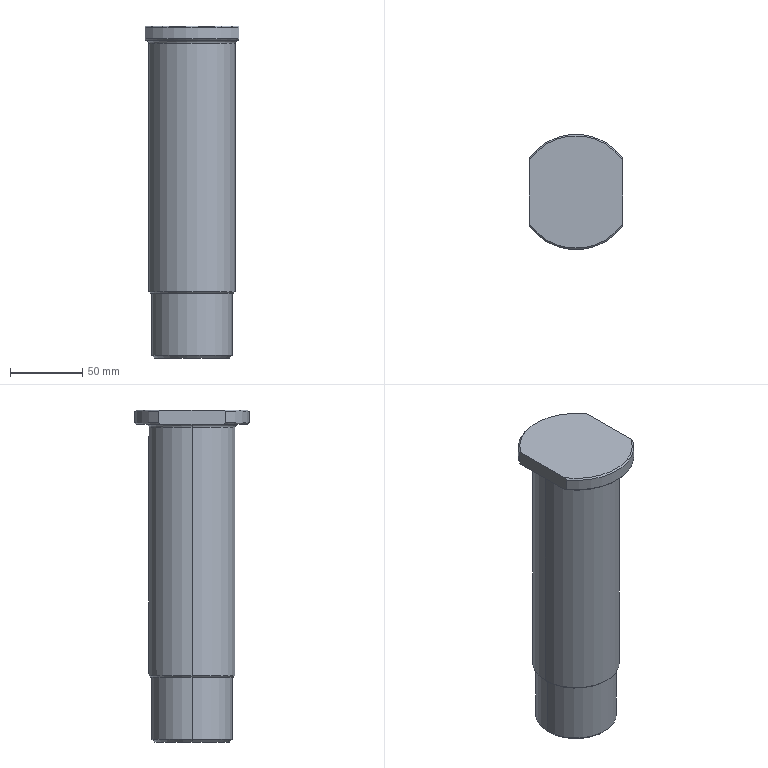Part | SolidWorks | features Chamfer 2, Fillet 2, ICE 2, Revolution 1 | 1 solid | 30 faces | box 65 x 80 x 230 mm | volume 649183 mm3 | cone 10 | cylinder 9 | plane 9 | torus 2 | commonest cylinder face diameters 56 x3 8 x2 60 x2 80 x2
STEP:
#1=CARTESIAN_POINT('',(-32.,0.,-10.));
#2=VERTEX_POINT('',#1);
#3=CARTESIAN_POINT('',(32.,0.,-10.));
#4=VERTEX_POINT('',#3);
#5=CARTESIAN_POINT('',(0.,0.,-10.));
#6=DIRECTION('',(0.,0.,1.));
#7=DIRECTION('',(1.,0.,0.));
#8=AXIS2_PLACEMENT_3D('',#5,#6,#7);
#9=CIRCLE('',#8,32.);
#10=EDGE_CURVE('',#2,#4,#9,.T.);
#11=ORIENTED_EDGE('',*,*,#10,.F.);
#12=CARTESIAN_POINT('',(-30.,0.,-12.));
#13=VERTEX_POINT('',#12);
#14=CARTESIAN_POINT('',(-32.,0.,-12.));
#15=DIRECTION('',(0.,1.,0.));
#16=DIRECTION('',(-1.,0.,0.));
#17=AXIS2_PLACEMENT_3D('',#14,#15,#16);
#18=CIRCLE('',#17,2.);
#19=EDGE_CURVE('',#2,#13,#18,.T.);
#20=ORIENTED_EDGE('',*,*,#19,.T.);
#21=CARTESIAN_POINT('',(30.,0.,-12.));
#22=VERTEX_POINT('',#21);
#23=CARTESIAN_POINT('',(0.,0.,-12.));
#24=DIRECTION('',(0.,0.,-1.));
#25=DIRECTION('',(1.,0.,0.));
#26=AXIS2_PLACEMENT_3D('',#23,#24,#25);
#27=CIRCLE('',#26,30.);
#28=EDGE_CURVE('',#22,#13,#27,.T.);
#29=ORIENTED_EDGE('',*,*,#28,.F.);
#30=CARTESIAN_POINT('',(32.,0.,-12.));
#31=DIRECTION('',(0.,-1.,0.));
#32=DIRECTION('',(0.,0.,-1.));
#33=AXIS2_PLACEMENT_3D('',#30,#31,#32);
#34=CIRCLE('',#33,2.);
#35=EDGE_CURVE('',#4,#22,#34,.T.);
#36=ORIENTED_EDGE('',*,*,#35,.F.);
#37=EDGE_LOOP('',(#11,#20,#29,#36));
#38=FACE_OUTER_BOUND('',#37,.T.);
#39=CARTESIAN_POINT('',(0.,0.,-12.));
#40=DIRECTION('',(0.,0.,1.));
#41=DIRECTION('',(1.,0.,0.));
#42=AXIS2_PLACEMENT_3D('',#39,#40,#41);
#43=TOROIDAL_SURFACE('',#42,32.,2.);
#44=ADVANCED_FACE('',(#38),#43,.F.);
#45=CARTESIAN_POINT('',(-26.,0.,-230.));
#46=VERTEX_POINT('',#45);
#47=CARTESIAN_POINT('',(-4.,25.69,-230.));
#48=VERTEX_POINT('',#47);
#49=CARTESIAN_POINT('',(0.,0.,-230.));
#50=DIRECTION('',(0.,0.,-1.));
#51=DIRECTION('',(1.,0.,0.));
#52=AXIS2_PLACEMENT_3D('',#49,#50,#51);
#53=CIRCLE('',#52,26.);
#54=EDGE_CURVE('',#46,#48,#53,.T.);
#55=ORIENTED_EDGE('',*,*,#54,.F.);
#56=CARTESIAN_POINT('',(-28.,0.,-228.));
#57=VERTEX_POINT('',#56);
#58=CARTESIAN_POINT('',(-28.,0.,-228.));
#59=DIRECTION('',(-0.7071,0.,0.7071));
#60=VECTOR('',#59,1000.);
#61=LINE('',#58,#60);
#62=EDGE_CURVE('',#46,#57,#61,.T.);
#63=ORIENTED_EDGE('',*,*,#62,.T.);
#64=CARTESIAN_POINT('',(-4.,27.713,-228.));
#65=VERTEX_POINT('',#64);
#66=CARTESIAN_POINT('',(0.,0.,-228.));
#67=DIRECTION('',(0.,0.,1.));
#68=DIRECTION('',(1.,0.,0.));
#69=AXIS2_PLACEMENT_3D('',#66,#67,#68);
#70=CIRCLE('',#69,28.);
#71=EDGE_CURVE('',#65,#57,#70,.T.);
#72=ORIENTED_EDGE('',*,*,#71,.F.);
#73=CARTESIAN_POINT('',(-4.,25.69,-230.));
#74=CARTESIAN_POINT('',(-4.,26.365,-229.334));
#75=CARTESIAN_POINT('',(-4.,27.039,-228.667));
#76=CARTESIAN_POINT('',(-4.,27.713,-228.));
#77=B_SPLINE_CURVE_WITH_KNOTS('',3,(#73,#74,#75,#76),.UNSPECIFIED.,.F.,.F.,(4,4),(0.006371,0.009215),.UNSPECIFIED.);
#78=EDGE_CURVE('',#48,#65,#77,.T.);
#79=ORIENTED_EDGE('',*,*,#78,.F.);
#80=EDGE_LOOP('',(#55,#63,#72,#79));
#81=FACE_OUTER_BOUND('',#80,.T.);
#82=CARTESIAN_POINT('',(0.,0.,-228.));
#83=DIRECTION('',(0.,0.,1.));
#84=DIRECTION('',(1.,0.,0.));
#85=AXIS2_PLACEMENT_3D('',#82,#83,#84);
#86=CONICAL_SURFACE('',#85,28.,0.7854);
#87=ADVANCED_FACE('',(#81),#86,.T.);
#88=ORIENTED_EDGE('',*,*,#62,.F.);
#89=CARTESIAN_POINT('',(26.,0.,-230.));
#90=VERTEX_POINT('',#89);
#91=CARTESIAN_POINT('',(0.,0.,-230.));
#92=DIRECTION('',(0.,0.,-1.));
#93=DIRECTION('',(1.,0.,0.));
#94=AXIS2_PLACEMENT_3D('',#91,#92,#93);
#95=CIRCLE('',#94,26.);
#96=EDGE_CURVE('',#90,#46,#95,.T.);
#97=ORIENTED_EDGE('',*,*,#96,.F.);
#98=CARTESIAN_POINT('',(28.,0.,-228.));
#99=VERTEX_POINT('',#98);
#100=CARTESIAN_POINT('',(28.,0.,-228.));
#101=DIRECTION('',(0.7071,0.,0.7071));
#102=VECTOR('',#101,1000.);
#103=LINE('',#100,#102);
#104=EDGE_CURVE('',#90,#99,#103,.T.);
#105=ORIENTED_EDGE('',*,*,#104,.T.);
#106=CARTESIAN_POINT('',(0.,0.,-228.));
#107=DIRECTION('',(0.,0.,1.));
#108=DIRECTION('',(1.,0.,0.));
#109=AXIS2_PLACEMENT_3D('',#106,#107,#108);
#110=CIRCLE('',#109,28.);
#111=EDGE_CURVE('',#57,#99,#110,.T.);
#112=ORIENTED_EDGE('',*,*,#111,.F.);
#113=EDGE_LOOP('',(#88,#97,#105,#112));
#114=FACE_OUTER_BOUND('',#113,.T.);
#115=CARTESIAN_POINT('',(0.,0.,-228.));
#116=DIRECTION('',(0.,0.,1.));
#117=DIRECTION('',(1.,0.,0.));
#118=AXIS2_PLACEMENT_3D('',#115,#116,#117);
#119=CONICAL_SURFACE('',#118,28.,0.7854);
#120=ADVANCED_FACE('',(#114),#119,.T.);
#121=CARTESIAN_POINT('',(-29.,0.,-185.));
#122=VERTEX_POINT('',#121);
#123=CARTESIAN_POINT('',(-4.,28.723,-185.));
#124=VERTEX_POINT('',#123);
#125=CARTESIAN_POINT('',(0.,0.,-185.));
#126=DIRECTION('',(0.,0.,-1.));
#127=DIRECTION('',(1.,0.,0.));
#128=AXIS2_PLACEMENT_3D('',#125,#126,#127);
#129=CIRCLE('',#128,29.);
#130=EDGE_CURVE('',#122,#124,#129,.T.);
#131=ORIENTED_EDGE('',*,*,#130,.F.);
#132=CARTESIAN_POINT('',(-30.,0.,-184.));
#133=VERTEX_POINT('',#132);
#134=CARTESIAN_POINT('',(-30.,0.,-184.));
#135=DIRECTION('',(-0.7071,0.,0.7071));
#136=VECTOR('',#135,1000.);
#137=LINE('',#134,#136);
#138=EDGE_CURVE('',#122,#133,#137,.T.);
#139=ORIENTED_EDGE('',*,*,#138,.T.);
#140=CARTESIAN_POINT('',(-3.873,29.749,-184.));
#141=VERTEX_POINT('',#140);
#142=CARTESIAN_POINT('',(0.,0.,-184.));
#143=DIRECTION('',(0.,0.,1.));
#144=DIRECTION('',(1.,0.,0.));
#145=AXIS2_PLACEMENT_3D('',#142,#143,#144);
#146=CIRCLE('',#145,30.);
#147=EDGE_CURVE('',#141,#133,#146,.T.);
#148=ORIENTED_EDGE('',*,*,#147,.F.);
#149=CARTESIAN_POINT('',(-3.873,29.749,-184.));
#150=CARTESIAN_POINT('',(-3.958,29.407,-184.328));
#151=CARTESIAN_POINT('',(-4.,29.065,-184.661));
#152=CARTESIAN_POINT('',(-4.,28.723,-185.));
#153=B_SPLINE_CURVE_WITH_KNOTS('',3,(#149,#150,#151,#152),.UNSPECIFIED.,.F.,.F.,(4,4),(0.,0.001438),.UNSPECIFIED.);
#154=EDGE_CURVE('',#141,#124,#153,.T.);
#155=ORIENTED_EDGE('',*,*,#154,.T.);
#156=EDGE_LOOP('',(#131,#139,#148,#155));
#157=FACE_OUTER_BOUND('',#156,.T.);
#158=CARTESIAN_POINT('',(0.,0.,-184.));
#159=DIRECTION('',(0.,0.,1.));
#160=DIRECTION('',(1.,0.,0.));
#161=AXIS2_PLACEMENT_3D('',#158,#159,#160);
#162=CONICAL_SURFACE('',#161,30.,0.7854);
#163=ADVANCED_FACE('',(#157),#162,.T.);
#164=ORIENTED_EDGE('',*,*,#138,.F.);
#165=CARTESIAN_POINT('',(29.,0.,-185.));
#166=VERTEX_POINT('',#165);
#167=CARTESIAN_POINT('',(0.,0.,-185.));
#168=DIRECTION('',(0.,0.,-1.));
#169=DIRECTION('',(1.,0.,0.));
#170=AXIS2_PLACEMENT_3D('',#167,#168,#169);
#171=CIRCLE('',#170,29.);
#172=EDGE_CURVE('',#166,#122,#171,.T.);
#173=ORIENTED_EDGE('',*,*,#172,.F.);
#174=CARTESIAN_POINT('',(30.,0.,-184.));
#175=VERTEX_POINT('',#174);
#176=CARTESIAN_POINT('',(30.,0.,-184.));
#177=DIRECTION('',(0.7071,0.,0.7071));
#178=VECTOR('',#177,1000.);
#179=LINE('',#176,#178);
#180=EDGE_CURVE('',#166,#175,#179,.T.);
#181=ORIENTED_EDGE('',*,*,#180,.T.);
#182=CARTESIAN_POINT('',(0.,0.,-184.));
#183=DIRECTION('',(0.,0.,1.));
#184=DIRECTION('',(1.,0.,0.));
#185=AXIS2_PLACEMENT_3D('',#182,#183,#184);
#186=CIRCLE('',#185,30.);
#187=EDGE_CURVE('',#133,#175,#186,.T.);
#188=ORIENTED_EDGE('',*,*,#187,.F.);
#189=EDGE_LOOP('',(#164,#173,#181,#188));
#190=FACE_OUTER_BOUND('',#189,.T.);
#191=CARTESIAN_POINT('',(0.,0.,-184.));
#192=DIRECTION('',(0.,0.,1.));
#193=DIRECTION('',(1.,0.,0.));
#194=AXIS2_PLACEMENT_3D('',#191,#192,#193);
#195=CONICAL_SURFACE('',#194,30.,0.7854);
#196=ADVANCED_FACE('',(#190),#195,.T.);
#197=ORIENTED_EDGE('',*,*,#147,.T.);
#198=CARTESIAN_POINT('',(-30.,0.,-10.));
#199=DIRECTION('',(0.,0.,1.));
#200=VECTOR('',#199,1000.);
#201=LINE('',#198,#200);
#202=EDGE_CURVE('',#133,#13,#201,.T.);
#203=ORIENTED_EDGE('',*,*,#202,.T.);
#204=CARTESIAN_POINT('',(0.,0.,-12.));
#205=DIRECTION('',(0.,0.,-1.));
#206=DIRECTION('',(1.,0.,0.));
#207=AXIS2_PLACEMENT_3D('',#204,#205,#206);
#208=CIRCLE('',#207,30.);
#209=EDGE_CURVE('',#13,#22,#208,.T.);
#210=ORIENTED_EDGE('',*,*,#209,.T.);
#211=CARTESIAN_POINT('',(30.,0.,-10.));
#212=DIRECTION('',(0.,0.,1.));
#213=VECTOR('',#212,1000.);
#214=LINE('',#211,#213);
#215=EDGE_CURVE('',#175,#22,#214,.T.);
#216=ORIENTED_EDGE('',*,*,#215,.F.);
#217=CARTESIAN_POINT('',(3.873,29.749,-184.));
#218=VERTEX_POINT('',#217);
#219=CARTESIAN_POINT('',(0.,0.,-184.));
#220=DIRECTION('',(0.,0.,1.));
#221=DIRECTION('',(1.,0.,0.));
#222=AXIS2_PLACEMENT_3D('',#219,#220,#221);
#223=CIRCLE('',#222,30.);
#224=EDGE_CURVE('',#175,#218,#223,.T.);
#225=ORIENTED_EDGE('',*,*,#224,.T.);
#226=CARTESIAN_POINT('',(0.,30.,-181.));
#227=VERTEX_POINT('',#226);
#228=CARTESIAN_POINT('',(3.873,29.749,-184.));
#229=CARTESIAN_POINT('',(3.762,29.763,-183.57));
#230=CARTESIAN_POINT('',(3.585,29.786,-183.171));
#231=CARTESIAN_POINT('',(3.098,29.841,-182.431));
#232=CARTESIAN_POINT('',(2.801,29.871,-182.11));
#233=CARTESIAN_POINT('',(2.102,29.928,-181.568));
#234=CARTESIAN_POINT('',(1.716,29.954,-181.36));
#235=CARTESIAN_POINT('',(1.089,29.981,-181.145));
#236=CARTESIAN_POINT('',(0.8739,29.988,-181.09));
#237=CARTESIAN_POINT('',(0.4412,29.998,-181.018));
#238=CARTESIAN_POINT('',(0.222,30.,-181.));
#239=CARTESIAN_POINT('',(0.,30.,-181.));
#240=B_SPLINE_CURVE_WITH_KNOTS('',3,(#228,#229,#230,#231,#232,#233,#234,#235,#236,#237,#238,#239),.UNSPECIFIED.,.F.,.F.,(4,2,2,2,2,4),(0.,0.001313,0.002626,0.003939,0.004596,0.005252),.UNSPECIFIED.);
#241=EDGE_CURVE('',#218,#227,#240,.T.);
#242=ORIENTED_EDGE('',*,*,#241,.T.);
#243=CARTESIAN_POINT('',(0.,30.,-181.));
#244=CARTESIAN_POINT('',(-0.444,30.,-181.));
#245=CARTESIAN_POINT('',(-0.8757,29.99,-181.072));
#246=CARTESIAN_POINT('',(-1.714,29.954,-181.359));
#247=CARTESIAN_POINT('',(-2.1,29.928,-181.567));
#248=CARTESIAN_POINT('',(-2.799,29.871,-182.108));
#249=CARTESIAN_POINT('',(-3.097,29.841,-182.43));
#250=CARTESIAN_POINT('',(-3.461,29.8,-182.983));
#251=CARTESIAN_POINT('',(-3.567,29.787,-183.177));
#252=CARTESIAN_POINT('',(-3.745,29.765,-183.578));
#253=CARTESIAN_POINT('',(-3.818,29.756,-183.785));
#254=CARTESIAN_POINT('',(-3.873,29.749,-184.));
#255=B_SPLINE_CURVE_WITH_KNOTS('',3,(#243,#244,#245,#246,#247,#248,#249,#250,#251,#252,#253,#254),.UNSPECIFIED.,.F.,.F.,(4,2,2,2,2,4),(0.,0.001313,0.002626,0.003939,0.004596,0.005252),.UNSPECIFIED.);
#256=EDGE_CURVE('',#227,#141,#255,.T.);
#257=ORIENTED_EDGE('',*,*,#256,.T.);
#258=EDGE_LOOP('',(#197,#203,#210,#216,#225,#242,#257));
#259=FACE_OUTER_BOUND('',#258,.T.);
#260=CARTESIAN_POINT('',(0.,0.,-10.));
#261=DIRECTION('',(0.,0.,1.));
#262=DIRECTION('',(1.,0.,0.));
#263=AXIS2_PLACEMENT_3D('',#260,#261,#262);
#264=CYLINDRICAL_SURFACE('',#263,30.);
#265=ADVANCED_FACE('',(#259),#264,.T.);
#266=ORIENTED_EDGE('',*,*,#71,.T.);
#267=CARTESIAN_POINT('',(-28.,0.,-185.));
#268=VERTEX_POINT('',#267);
#269=CARTESIAN_POINT('',(-28.,0.,-10.));
#270=DIRECTION('',(0.,0.,1.));
#271=VECTOR('',#270,1000.);
#272=LINE('',#269,#271);
#273=EDGE_CURVE('',#57,#268,#272,.T.);
#274=ORIENTED_EDGE('',*,*,#273,.T.);
#275=CARTESIAN_POINT('',(-4.,27.713,-185.));
#276=VERTEX_POINT('',#275);
#277=CARTESIAN_POINT('',(0.,0.,-185.));
#278=DIRECTION('',(0.,0.,1.));
#279=DIRECTION('',(1.,0.,0.));
#280=AXIS2_PLACEMENT_3D('',#277,#278,#279);
#281=CIRCLE('',#280,28.);
#282=EDGE_CURVE('',#276,#268,#281,.T.);
#283=ORIENTED_EDGE('',*,*,#282,.F.);
#284=CARTESIAN_POINT('',(-4.,27.713,-10.));
#285=DIRECTION('',(0.,0.,1.));
#286=VECTOR('',#285,1000.);
#287=LINE('',#284,#286);
#288=EDGE_CURVE('',#65,#276,#287,.T.);
#289=ORIENTED_EDGE('',*,*,#288,.F.);
#290=EDGE_LOOP('',(#266,#274,#283,#289));
#291=FACE_OUTER_BOUND('',#290,.T.);
#292=CARTESIAN_POINT('',(0.,0.,-10.));
#293=DIRECTION('',(0.,0.,1.));
#294=DIRECTION('',(1.,0.,0.));
#295=AXIS2_PLACEMENT_3D('',#292,#293,#294);
#296=CYLINDRICAL_SURFACE('',#295,28.);
#297=ADVANCED_FACE('',(#291),#296,.T.);
#298=ORIENTED_EDGE('',*,*,#273,.F.);
#299=ORIENTED_EDGE('',*,*,#111,.T.);
#300=CARTESIAN_POINT('',(28.,0.,-185.));
#301=VERTEX_POINT('',#300);
#302=CARTESIAN_POINT('',(28.,0.,-10.));
#303=DIRECTION('',(0.,0.,1.));
#304=VECTOR('',#303,1000.);
#305=LINE('',#302,#304);
#306=EDGE_CURVE('',#99,#301,#305,.T.);
#307=ORIENTED_EDGE('',*,*,#306,.T.);
#308=CARTESIAN_POINT('',(0.,0.,-185.));
#309=DIRECTION('',(0.,0.,1.));
#310=DIRECTION('',(1.,0.,0.));
#311=AXIS2_PLACEMENT_3D('',#308,#309,#310);
#312=CIRCLE('',#311,28.);
#313=EDGE_CURVE('',#268,#301,#312,.T.);
#314=ORIENTED_EDGE('',*,*,#313,.F.);
#315=EDGE_LOOP('',(#298,#299,#307,#314));
#316=FACE_OUTER_BOUND('',#315,.T.);
#317=CARTESIAN_POINT('',(0.,0.,-10.));
#318=DIRECTION('',(0.,0.,1.));
#319=DIRECTION('',(1.,0.,0.));
#320=AXIS2_PLACEMENT_3D('',#317,#318,#319);
#321=CYLINDRICAL_SURFACE('',#320,28.);
#322=ADVANCED_FACE('',(#316),#321,.T.);
#323=CARTESIAN_POINT('',(0.,0.,-10.));
#324=DIRECTION('',(0.,0.,1.));
#325=DIRECTION('',(1.,0.,0.));
#326=AXIS2_PLACEMENT_3D('',#323,#324,#325);
#327=CIRCLE('',#326,32.);
#328=EDGE_CURVE('',#4,#2,#327,.T.);
#329=ORIENTED_EDGE('',*,*,#328,.T.);
#330=ORIENTED_EDGE('',*,*,#10,.T.);
#331=EDGE_LOOP('',(#329,#330));
#332=FACE_BOUND('',#331,.T.);
#333=CARTESIAN_POINT('',(32.5,-21.558,-10.));
#334=VERTEX_POINT('',#333);
#335=CARTESIAN_POINT('',(-32.5,-21.558,-10.));
#336=VERTEX_POINT('',#335);
#337=CARTESIAN_POINT('',(0.,0.,-10.));
#338=DIRECTION('',(0.,0.,-1.));
#339=DIRECTION('',(1.,0.,0.));
#340=AXIS2_PLACEMENT_3D('',#337,#338,#339);
#341=CIRCLE('',#340,39.);
#342=EDGE_CURVE('',#334,#336,#341,.T.);
#343=ORIENTED_EDGE('',*,*,#342,.T.);
#344=CARTESIAN_POINT('',(-32.5,21.558,-10.));
#345=VERTEX_POINT('',#344);
#346=CARTESIAN_POINT('',(-32.5,0.,-10.));
#347=DIRECTION('',(0.,1.,0.));
#348=VECTOR('',#347,1000.);
#349=LINE('',#346,#348);
#350=EDGE_CURVE('',#336,#345,#349,.T.);
#351=ORIENTED_EDGE('',*,*,#350,.T.);
#352=CARTESIAN_POINT('',(32.5,21.558,-10.));
#353=VERTEX_POINT('',#352);
#354=CARTESIAN_POINT('',(0.,0.,-10.));
#355=DIRECTION('',(0.,0.,-1.));
#356=DIRECTION('',(1.,0.,0.));
#357=AXIS2_PLACEMENT_3D('',#354,#355,#356);
#358=CIRCLE('',#357,39.);
#359=EDGE_CURVE('',#345,#353,#358,.T.);
#360=ORIENTED_EDGE('',*,*,#359,.T.);
#361=CARTESIAN_POINT('',(32.5,0.,-10.));
#362=DIRECTION('',(0.,1.,0.));
#363=VECTOR('',#362,1000.);
#364=LINE('',#361,#363);
#365=EDGE_CURVE('',#334,#353,#364,.T.);
#366=ORIENTED_EDGE('',*,*,#365,.F.);
#367=EDGE_LOOP('',(#343,#351,#360,#366));
#368=FACE_OUTER_BOUND('',#367,.T.);
#369=CARTESIAN_POINT('',(0.,0.,-10.));
#370=DIRECTION('',(0.,0.,1.));
#371=DIRECTION('',(1.,0.,0.));
#372=AXIS2_PLACEMENT_3D('',#369,#370,#371);
#373=PLANE('',#372);
#374=ADVANCED_FACE('',(#332,#368),#373,.F.);
#375=CARTESIAN_POINT('',(-32.5,23.318,-1.));
#376=VERTEX_POINT('',#375);
#377=CARTESIAN_POINT('',(-32.5,23.318,-9.));
#378=VERTEX_POINT('',#377);
#379=CARTESIAN_POINT('',(-32.5,23.318,-10.));
#380=DIRECTION('',(0.,0.,-1.));
#381=VECTOR('',#380,1000.);
#382=LINE('',#379,#381);
#383=EDGE_CURVE('',#376,#378,#382,.T.);
#384=ORIENTED_EDGE('',*,*,#383,.F.);
#385=CARTESIAN_POINT('',(32.5,23.318,-1.));
#386=VERTEX_POINT('',#385);
#387=CARTESIAN_POINT('',(0.,0.,-1.));
#388=DIRECTION('',(0.,0.,-1.));
#389=DIRECTION('',(1.,0.,0.));
#390=AXIS2_PLACEMENT_3D('',#387,#388,#389);
#391=CIRCLE('',#390,40.);
#392=EDGE_CURVE('',#376,#386,#391,.T.);
#393=ORIENTED_EDGE('',*,*,#392,.T.);
#394=CARTESIAN_POINT('',(32.5,23.318,-9.));
#395=VERTEX_POINT('',#394);
#396=CARTESIAN_POINT('',(32.5,23.318,-10.));
#397=DIRECTION('',(0.,0.,-1.));
#398=VECTOR('',#397,1000.);
#399=LINE('',#396,#398);
#400=EDGE_CURVE('',#386,#395,#399,.T.);
#401=ORIENTED_EDGE('',*,*,#400,.T.);
#402=CARTESIAN_POINT('',(0.,0.,-9.));
#403=DIRECTION('',(0.,0.,1.));
#404=DIRECTION('',(1.,0.,0.));
#405=AXIS2_PLACEMENT_3D('',#402,#403,#404);
#406=CIRCLE('',#405,40.);
#407=EDGE_CURVE('',#395,#378,#406,.T.);
#408=ORIENTED_EDGE('',*,*,#407,.T.);
#409=EDGE_LOOP('',(#384,#393,#401,#408));
#410=FACE_OUTER_BOUND('',#409,.T.);
#411=CARTESIAN_POINT('',(0.,0.,-10.));
#412=DIRECTION('',(0.,0.,1.));
#413=DIRECTION('',(1.,0.,0.));
#414=AXIS2_PLACEMENT_3D('',#411,#412,#413);
#415=CYLINDRICAL_SURFACE('',#414,40.);
#416=ADVANCED_FACE('',(#410),#415,.T.);
#417=CARTESIAN_POINT('',(-32.5,-23.318,-9.));
#418=VERTEX_POINT('',#417);
#419=CARTESIAN_POINT('',(-32.5,-23.318,-1.));
#420=VERTEX_POINT('',#419);
#421=CARTESIAN_POINT('',(-32.5,-23.318,-10.));
#422=DIRECTION('',(0.,0.,1.));
#423=VECTOR('',#422,1000.);
#424=LINE('',#421,#423);
#425=EDGE_CURVE('',#418,#420,#424,.T.);
#426=ORIENTED_EDGE('',*,*,#425,.F.);
#427=CARTESIAN_POINT('',(32.5,-23.318,-9.));
#428=VERTEX_POINT('',#427);
#429=CARTESIAN_POINT('',(0.,0.,-9.));
#430=DIRECTION('',(0.,0.,1.));
#431=DIRECTION('',(1.,0.,0.));
#432=AXIS2_PLACEMENT_3D('',#429,#430,#431);
#433=CIRCLE('',#432,40.);
#434=EDGE_CURVE('',#418,#428,#433,.T.);
#435=ORIENTED_EDGE('',*,*,#434,.T.);
#436=CARTESIAN_POINT('',(32.5,-23.318,-1.));
#437=VERTEX_POINT('',#436);
#438=CARTESIAN_POINT('',(32.5,-23.318,-10.));
#439=DIRECTION('',(0.,0.,1.));
#440=VECTOR('',#439,1000.);
#441=LINE('',#438,#440);
#442=EDGE_CURVE('',#428,#437,#441,.T.);
#443=ORIENTED_EDGE('',*,*,#442,.T.);
#444=CARTESIAN_POINT('',(0.,0.,-1.));
#445=DIRECTION('',(0.,0.,-1.));
#446=DIRECTION('',(1.,0.,0.));
#447=AXIS2_PLACEMENT_3D('',#444,#445,#446);
#448=CIRCLE('',#447,40.);
#449=EDGE_CURVE('',#437,#420,#448,.T.);
#450=ORIENTED_EDGE('',*,*,#449,.T.);
#451=EDGE_LOOP('',(#426,#435,#443,#450));
#452=FACE_OUTER_BOUND('',#451,.T.);
#453=CARTESIAN_POINT('',(0.,0.,-10.));
#454=DIRECTION('',(0.,0.,1.));
#455=DIRECTION('',(1.,0.,0.));
#456=AXIS2_PLACEMENT_3D('',#453,#454,#455);
#457=CYLINDRICAL_SURFACE('',#456,40.);
#458=ADVANCED_FACE('',(#452),#457,.T.);
#459=CARTESIAN_POINT('',(-32.5,-21.558,0.));
#460=VERTEX_POINT('',#459);
#461=CARTESIAN_POINT('',(-32.5,21.558,0.));
#462=VERTEX_POINT('',#461);
#463=CARTESIAN_POINT('',(-32.5,0.,0.));
#464=DIRECTION('',(0.,1.,0.));
#465=VECTOR('',#464,1000.);
#466=LINE('',#463,#465);
#467=EDGE_CURVE('',#460,#462,#466,.T.);
#468=ORIENTED_EDGE('',*,*,#467,.F.);
#469=CARTESIAN_POINT('',(32.5,-21.558,0.));
#470=VERTEX_POINT('',#469);
#471=CARTESIAN_POINT('',(0.,0.,0.));
#472=DIRECTION('',(0.,0.,1.));
#473=DIRECTION('',(1.,0.,0.));
#474=AXIS2_PLACEMENT_3D('',#471,#472,#473);
#475=CIRCLE('',#474,39.);
#476=EDGE_CURVE('',#460,#470,#475,.T.);
#477=ORIENTED_EDGE('',*,*,#476,.T.);
#478=CARTESIAN_POINT('',(32.5,21.558,0.));
#479=VERTEX_POINT('',#478);
#480=CARTESIAN_POINT('',(32.5,0.,0.));
#481=DIRECTION('',(0.,1.,0.));
#482=VECTOR('',#481,1000.);
#483=LINE('',#480,#482);
#484=EDGE_CURVE('',#470,#479,#483,.T.);
#485=ORIENTED_EDGE('',*,*,#484,.T.);
#486=CARTESIAN_POINT('',(0.,0.,0.));
#487=DIRECTION('',(0.,0.,1.));
#488=DIRECTION('',(1.,0.,0.));
#489=AXIS2_PLACEMENT_3D('',#486,#487,#488);
#490=CIRCLE('',#489,39.);
#491=EDGE_CURVE('',#479,#462,#490,.T.);
#492=ORIENTED_EDGE('',*,*,#491,.T.);
#493=EDGE_LOOP('',(#468,#477,#485,#492));
#494=FACE_OUTER_BOUND('',#493,.T.);
#495=CARTESIAN_POINT('',(0.,0.,0.));
#496=DIRECTION('',(0.,0.,1.));
#497=DIRECTION('',(1.,0.,0.));
#498=AXIS2_PLACEMENT_3D('',#495,#496,#497);
#499=PLANE('',#498);
#500=ADVANCED_FACE('',(#494),#499,.T.);
#501=CARTESIAN_POINT('',(-32.5,-23.318,-1.));
#502=CARTESIAN_POINT('',(-32.5,-22.735,-0.6597));
#503=CARTESIAN_POINT('',(-32.5,-22.148,-0.3261));
#504=CARTESIAN_POINT('',(-32.5,-21.558,0.));
#505=B_SPLINE_CURVE_WITH_KNOTS('',3,(#501,#502,#503,#504),.UNSPECIFIED.,.F.,.F.,(4,4),(0.000001379,0.002013),.UNSPECIFIED.);
#506=EDGE_CURVE('',#420,#460,#505,.T.);
#507=ORIENTED_EDGE('',*,*,#506,.F.);
#508=ORIENTED_EDGE('',*,*,#449,.F.);
#509=CARTESIAN_POINT('',(32.5,-23.318,-1.));
#510=CARTESIAN_POINT('',(32.5,-22.735,-0.6597));
#511=CARTESIAN_POINT('',(32.5,-22.148,-0.3261));
#512=CARTESIAN_POINT('',(32.5,-21.558,0.));
#513=B_SPLINE_CURVE_WITH_KNOTS('',3,(#509,#510,#511,#512),.UNSPECIFIED.,.F.,.F.,(4,4),(0.000001379,0.002013),.UNSPECIFIED.);
#514=EDGE_CURVE('',#437,#470,#513,.T.);
#515=ORIENTED_EDGE('',*,*,#514,.T.);
#516=ORIENTED_EDGE('',*,*,#476,.F.);
#517=EDGE_LOOP('',(#507,#508,#515,#516));
#518=FACE_OUTER_BOUND('',#517,.T.);
#519=CARTESIAN_POINT('',(0.,0.,0.));
#520=DIRECTION('',(0.,0.,-1.));
#521=DIRECTION('',(-1.,0.,0.));
#522=AXIS2_PLACEMENT_3D('',#519,#520,#521);
#523=CONICAL_SURFACE('',#522,39.,0.7854);
#524=ADVANCED_FACE('',(#518),#523,.T.);
#525=CARTESIAN_POINT('',(-32.5,21.558,0.));
#526=CARTESIAN_POINT('',(-32.5,22.148,-0.3263));
#527=CARTESIAN_POINT('',(-32.5,22.735,-0.6599));
#528=CARTESIAN_POINT('',(-32.5,23.318,-1.));
#529=B_SPLINE_CURVE_WITH_KNOTS('',3,(#525,#526,#527,#528),.UNSPECIFIED.,.F.,.F.,(4,4),(0.04728,0.04929),.UNSPECIFIED.);
#530=EDGE_CURVE('',#462,#376,#529,.T.);
#531=ORIENTED_EDGE('',*,*,#530,.F.);
#532=ORIENTED_EDGE('',*,*,#491,.F.);
#533=CARTESIAN_POINT('',(32.5,21.558,0.));
#534=CARTESIAN_POINT('',(32.5,22.148,-0.3263));
#535=CARTESIAN_POINT('',(32.5,22.735,-0.6599));
#536=CARTESIAN_POINT('',(32.5,23.318,-1.));
#537=B_SPLINE_CURVE_WITH_KNOTS('',3,(#533,#534,#535,#536),.UNSPECIFIED.,.F.,.F.,(4,4),(0.04728,0.04929),.UNSPECIFIED.);
#538=EDGE_CURVE('',#479,#386,#537,.T.);
#539=ORIENTED_EDGE('',*,*,#538,.T.);
#540=ORIENTED_EDGE('',*,*,#392,.F.);
#541=EDGE_LOOP('',(#531,#532,#539,#540));
#542=FACE_OUTER_BOUND('',#541,.T.);
#543=CARTESIAN_POINT('',(0.,0.,0.));
#544=DIRECTION('',(0.,0.,-1.));
#545=DIRECTION('',(-1.,0.,0.));
#546=AXIS2_PLACEMENT_3D('',#543,#544,#545);
#547=CONICAL_SURFACE('',#546,39.,0.7854);
#548=ADVANCED_FACE('',(#542),#547,.T.);
#549=CARTESIAN_POINT('',(-32.5,23.318,-9.));
#550=CARTESIAN_POINT('',(-32.5,22.735,-9.34));
#551=CARTESIAN_POINT('',(-32.5,22.148,-9.674));
#552=CARTESIAN_POINT('',(-32.5,21.558,-10.));
#553=B_SPLINE_CURVE_WITH_KNOTS('',3,(#549,#550,#551,#552),.UNSPECIFIED.,.F.,.F.,(4,4),(0.000001379,0.002013),.UNSPECIFIED.);
#554=EDGE_CURVE('',#378,#345,#553,.T.);
#555=ORIENTED_EDGE('',*,*,#554,.F.);
#556=ORIENTED_EDGE('',*,*,#407,.F.);
#557=CARTESIAN_POINT('',(32.5,23.318,-9.));
#558=CARTESIAN_POINT('',(32.5,22.735,-9.34));
#559=CARTESIAN_POINT('',(32.5,22.148,-9.674));
#560=CARTESIAN_POINT('',(32.5,21.558,-10.));
#561=B_SPLINE_CURVE_WITH_KNOTS('',3,(#557,#558,#559,#560),.UNSPECIFIED.,.F.,.F.,(4,4),(0.000001379,0.002013),.UNSPECIFIED.);
#562=EDGE_CURVE('',#395,#353,#561,.T.);
#563=ORIENTED_EDGE('',*,*,#562,.T.);
#564=ORIENTED_EDGE('',*,*,#359,.F.);
#565=EDGE_LOOP('',(#555,#556,#563,#564));
#566=FACE_OUTER_BOUND('',#565,.T.);
#567=CARTESIAN_POINT('',(0.,0.,-9.));
#568=DIRECTION('',(0.,0.,1.));
#569=DIRECTION('',(1.,0.,0.));
#570=AXIS2_PLACEMENT_3D('',#567,#568,#569);
#571=CONICAL_SURFACE('',#570,40.,0.7854);
#572=ADVANCED_FACE('',(#566),#571,.T.);
#573=CARTESIAN_POINT('',(-32.5,-21.558,-10.));
#574=CARTESIAN_POINT('',(-32.5,-22.148,-9.674));
#575=CARTESIAN_POINT('',(-32.5,-22.735,-9.34));
#576=CARTESIAN_POINT('',(-32.5,-23.318,-9.));
#577=B_SPLINE_CURVE_WITH_KNOTS('',3,(#573,#574,#575,#576),.UNSPECIFIED.,.F.,.F.,(4,4),(0.04728,0.04929),.UNSPECIFIED.);
#578=EDGE_CURVE('',#336,#418,#577,.T.);
#579=ORIENTED_EDGE('',*,*,#578,.F.);
#580=ORIENTED_EDGE('',*,*,#342,.F.);
#581=CARTESIAN_POINT('',(32.5,-21.558,-10.));
#582=CARTESIAN_POINT('',(32.5,-22.148,-9.674));
#583=CARTESIAN_POINT('',(32.5,-22.735,-9.34));
#584=CARTESIAN_POINT('',(32.5,-23.318,-9.));
#585=B_SPLINE_CURVE_WITH_KNOTS('',3,(#581,#582,#583,#584),.UNSPECIFIED.,.F.,.F.,(4,4),(0.04728,0.04929),.UNSPECIFIED.);
#586=EDGE_CURVE('',#334,#428,#585,.T.);
#587=ORIENTED_EDGE('',*,*,#586,.T.);
#588=ORIENTED_EDGE('',*,*,#434,.F.);
#589=EDGE_LOOP('',(#579,#580,#587,#588));
#590=FACE_OUTER_BOUND('',#589,.T.);
#591=CARTESIAN_POINT('',(0.,0.,-9.));
#592=DIRECTION('',(0.,0.,1.));
#593=DIRECTION('',(1.,0.,0.));
#594=AXIS2_PLACEMENT_3D('',#591,#592,#593);
#595=CONICAL_SURFACE('',#594,40.,0.7854);
#596=ADVANCED_FACE('',(#590),#595,.T.);
#597=CARTESIAN_POINT('',(4.,24.,-230.));
#598=VERTEX_POINT('',#597);
#599=CARTESIAN_POINT('',(4.,25.69,-230.));
#600=VERTEX_POINT('',#599);
#601=CARTESIAN_POINT('',(4.,24.,-230.));
#602=DIRECTION('',(0.,1.,0.));
#603=VECTOR('',#602,1000.);
#604=LINE('',#601,#603);
#605=EDGE_CURVE('',#598,#600,#604,.T.);
#606=ORIENTED_EDGE('',*,*,#605,.T.);
#607=CARTESIAN_POINT('',(0.,0.,-230.));
#608=DIRECTION('',(0.,0.,-1.));
#609=DIRECTION('',(1.,0.,0.));
#610=AXIS2_PLACEMENT_3D('',#607,#608,#609);
#611=CIRCLE('',#610,26.);
#612=EDGE_CURVE('',#600,#90,#611,.T.);
#613=ORIENTED_EDGE('',*,*,#612,.T.);
#614=ORIENTED_EDGE('',*,*,#96,.T.);
#615=ORIENTED_EDGE('',*,*,#54,.T.);
#616=CARTESIAN_POINT('',(-4.,24.,-230.));
#617=VERTEX_POINT('',#616);
#618=CARTESIAN_POINT('',(-4.,24.,-230.));
#619=DIRECTION('',(0.,1.,0.));
#620=VECTOR('',#619,1000.);
#621=LINE('',#618,#620);
#622=EDGE_CURVE('',#617,#48,#621,.T.);
#623=ORIENTED_EDGE('',*,*,#622,.F.);
#624=CARTESIAN_POINT('',(4.,24.,-230.));
#625=DIRECTION('',(-1.,0.,0.));
#626=VECTOR('',#625,1000.);
#627=LINE('',#624,#626);
#628=EDGE_CURVE('',#598,#617,#627,.T.);
#629=ORIENTED_EDGE('',*,*,#628,.F.);
#630=EDGE_LOOP('',(#606,#613,#614,#615,#623,#629));
#631=FACE_OUTER_BOUND('',#630,.T.);
#632=CARTESIAN_POINT('',(0.,0.,-230.));
#633=DIRECTION('',(0.,0.,1.));
#634=DIRECTION('',(1.,0.,0.));
#635=AXIS2_PLACEMENT_3D('',#632,#633,#634);
#636=PLANE('',#635);
#637=ADVANCED_FACE('',(#631),#636,.F.);
#638=ORIENTED_EDGE('',*,*,#306,.F.);
#639=CARTESIAN_POINT('',(4.,27.713,-228.));
#640=VERTEX_POINT('',#639);
#641=CARTESIAN_POINT('',(0.,0.,-228.));
#642=DIRECTION('',(0.,0.,1.));
#643=DIRECTION('',(1.,0.,0.));
#644=AXIS2_PLACEMENT_3D('',#641,#642,#643);
#645=CIRCLE('',#644,28.);
#646=EDGE_CURVE('',#99,#640,#645,.T.);
#647=ORIENTED_EDGE('',*,*,#646,.T.);
#648=CARTESIAN_POINT('',(4.,27.713,-185.));
#649=VERTEX_POINT('',#648);
#650=CARTESIAN_POINT('',(4.,27.713,-10.));
#651=DIRECTION('',(0.,0.,1.));
#652=VECTOR('',#651,1000.);
#653=LINE('',#650,#652);
#654=EDGE_CURVE('',#640,#649,#653,.T.);
#655=ORIENTED_EDGE('',*,*,#654,.T.);
#656=CARTESIAN_POINT('',(0.,0.,-185.));
#657=DIRECTION('',(0.,0.,1.));
#658=DIRECTION('',(1.,0.,0.));
#659=AXIS2_PLACEMENT_3D('',#656,#657,#658);
#660=CIRCLE('',#659,28.);
#661=EDGE_CURVE('',#301,#649,#660,.T.);
#662=ORIENTED_EDGE('',*,*,#661,.F.);
#663=EDGE_LOOP('',(#638,#647,#655,#662));
#664=FACE_OUTER_BOUND('',#663,.T.);
#665=CARTESIAN_POINT('',(0.,0.,-10.));
#666=DIRECTION('',(0.,0.,1.));
#667=DIRECTION('',(1.,0.,0.));
#668=AXIS2_PLACEMENT_3D('',#665,#666,#667);
#669=CYLINDRICAL_SURFACE('',#668,28.);
#670=ADVANCED_FACE('',(#664),#669,.T.);
#671=CARTESIAN_POINT('',(4.,28.723,-185.));
#672=VERTEX_POINT('',#671);
#673=CARTESIAN_POINT('',(4.,0.,-185.));
#674=DIRECTION('',(0.,-1.,0.));
#675=VECTOR('',#674,1000.);
#676=LINE('',#673,#675);
#677=EDGE_CURVE('',#672,#649,#676,.T.);
#678=ORIENTED_EDGE('',*,*,#677,.F.);
#679=CARTESIAN_POINT('',(0.,0.,-185.));
#680=DIRECTION('',(0.,0.,-1.));
#681=DIRECTION('',(1.,0.,0.));
#682=AXIS2_PLACEMENT_3D('',#679,#680,#681);
#683=CIRCLE('',#682,29.);
#684=EDGE_CURVE('',#672,#166,#683,.T.);
#685=ORIENTED_EDGE('',*,*,#684,.T.);
#686=ORIENTED_EDGE('',*,*,#172,.T.);
#687=ORIENTED_EDGE('',*,*,#130,.T.);
#688=CARTESIAN_POINT('',(-4.,0.,-185.));
#689=DIRECTION('',(0.,-1.,0.));
#690=VECTOR('',#689,1000.);
#691=LINE('',#688,#690);
#692=EDGE_CURVE('',#124,#276,#691,.T.);
#693=ORIENTED_EDGE('',*,*,#692,.T.);
#694=ORIENTED_EDGE('',*,*,#282,.T.);
#695=ORIENTED_EDGE('',*,*,#313,.T.);
#696=ORIENTED_EDGE('',*,*,#661,.T.);
#697=EDGE_LOOP('',(#678,#685,#686,#687,#693,#694,#695,#696));
#698=FACE_OUTER_BOUND('',#697,.T.);
#699=CARTESIAN_POINT('',(0.,0.,-185.));
#700=DIRECTION('',(0.,0.,1.));
#701=DIRECTION('',(1.,0.,0.));
#702=AXIS2_PLACEMENT_3D('',#699,#700,#701);
#703=PLANE('',#702);
#704=ADVANCED_FACE('',(#698),#703,.F.);
#705=ORIENTED_EDGE('',*,*,#202,.F.);
#706=ORIENTED_EDGE('',*,*,#187,.T.);
#707=ORIENTED_EDGE('',*,*,#215,.T.);
#708=ORIENTED_EDGE('',*,*,#28,.T.);
#709=EDGE_LOOP('',(#705,#706,#707,#708));
#710=FACE_OUTER_BOUND('',#709,.T.);
#711=CARTESIAN_POINT('',(0.,0.,-10.));
#712=DIRECTION('',(0.,0.,1.));
#713=DIRECTION('',(1.,0.,0.));
#714=AXIS2_PLACEMENT_3D('',#711,#712,#713);
#715=CYLINDRICAL_SURFACE('',#714,30.);
#716=ADVANCED_FACE('',(#710),#715,.T.);
#717=ORIENTED_EDGE('',*,*,#180,.F.);
#718=ORIENTED_EDGE('',*,*,#684,.F.);
#719=CARTESIAN_POINT('',(4.,28.723,-185.));
#720=CARTESIAN_POINT('',(4.,29.065,-184.661));
#721=CARTESIAN_POINT('',(3.958,29.407,-184.328));
#722=CARTESIAN_POINT('',(3.873,29.749,-184.));
#723=B_SPLINE_CURVE_WITH_KNOTS('',3,(#719,#720,#721,#722),.UNSPECIFIED.,.F.,.F.,(4,4),(0.,0.001438),.UNSPECIFIED.);
#724=EDGE_CURVE('',#672,#218,#723,.T.);
#725=ORIENTED_EDGE('',*,*,#724,.T.);
#726=ORIENTED_EDGE('',*,*,#224,.F.);
#727=EDGE_LOOP('',(#717,#718,#725,#726));
#728=FACE_OUTER_BOUND('',#727,.T.);
#729=CARTESIAN_POINT('',(0.,0.,-184.));
#730=DIRECTION('',(0.,0.,1.));
#731=DIRECTION('',(1.,0.,0.));
#732=AXIS2_PLACEMENT_3D('',#729,#730,#731);
#733=CONICAL_SURFACE('',#732,30.,0.7854);
#734=ADVANCED_FACE('',(#728),#733,.T.);
#735=ORIENTED_EDGE('',*,*,#104,.F.);
#736=ORIENTED_EDGE('',*,*,#612,.F.);
#737=CARTESIAN_POINT('',(4.,25.69,-230.));
#738=CARTESIAN_POINT('',(4.,26.365,-229.334));
#739=CARTESIAN_POINT('',(4.,27.039,-228.667));
#740=CARTESIAN_POINT('',(4.,27.713,-228.));
#741=B_SPLINE_CURVE_WITH_KNOTS('',3,(#737,#738,#739,#740),.UNSPECIFIED.,.F.,.F.,(4,4),(0.006371,0.009215),.UNSPECIFIED.);
#742=EDGE_CURVE('',#600,#640,#741,.T.);
#743=ORIENTED_EDGE('',*,*,#742,.T.);
#744=ORIENTED_EDGE('',*,*,#646,.F.);
#745=EDGE_LOOP('',(#735,#736,#743,#744));
#746=FACE_OUTER_BOUND('',#745,.T.);
#747=CARTESIAN_POINT('',(0.,0.,-228.));
#748=DIRECTION('',(0.,0.,1.));
#749=DIRECTION('',(1.,0.,0.));
#750=AXIS2_PLACEMENT_3D('',#747,#748,#749);
#751=CONICAL_SURFACE('',#750,28.,0.7854);
#752=ADVANCED_FACE('',(#746),#751,.T.);
#753=ORIENTED_EDGE('',*,*,#19,.F.);
#754=ORIENTED_EDGE('',*,*,#328,.F.);
#755=ORIENTED_EDGE('',*,*,#35,.T.);
#756=ORIENTED_EDGE('',*,*,#209,.F.);
#757=EDGE_LOOP('',(#753,#754,#755,#756));
#758=FACE_OUTER_BOUND('',#757,.T.);
#759=CARTESIAN_POINT('',(0.,0.,-12.));
#760=DIRECTION('',(0.,0.,1.));
#761=DIRECTION('',(1.,0.,0.));
#762=AXIS2_PLACEMENT_3D('',#759,#760,#761);
#763=TOROIDAL_SURFACE('',#762,32.,2.);
#764=ADVANCED_FACE('',(#758),#763,.F.);
#765=CARTESIAN_POINT('',(-4.,24.,-185.));
#766=VERTEX_POINT('',#765);
#767=CARTESIAN_POINT('',(0.,24.,-181.));
#768=VERTEX_POINT('',#767);
#769=CARTESIAN_POINT('',(0.,24.,-185.));
#770=DIRECTION('',(0.,1.,0.));
#771=DIRECTION('',(0.,0.,-1.));
#772=AXIS2_PLACEMENT_3D('',#769,#770,#771);
#773=CIRCLE('',#772,4.);
#774=EDGE_CURVE('',#766,#768,#773,.T.);
#775=ORIENTED_EDGE('',*,*,#774,.T.);
#776=CARTESIAN_POINT('',(4.,24.,-185.));
#777=VERTEX_POINT('',#776);
#778=CARTESIAN_POINT('',(0.,24.,-185.));
#779=DIRECTION('',(0.,1.,0.));
#780=DIRECTION('',(0.,0.,-1.));
#781=AXIS2_PLACEMENT_3D('',#778,#779,#780);
#782=CIRCLE('',#781,4.);
#783=EDGE_CURVE('',#768,#777,#782,.T.);
#784=ORIENTED_EDGE('',*,*,#783,.T.);
#785=CARTESIAN_POINT('',(4.,24.,-181.));
#786=DIRECTION('',(0.,0.,-1.));
#787=VECTOR('',#786,1000.);
#788=LINE('',#785,#787);
#789=EDGE_CURVE('',#777,#598,#788,.T.);
#790=ORIENTED_EDGE('',*,*,#789,.T.);
#791=ORIENTED_EDGE('',*,*,#628,.T.);
#792=CARTESIAN_POINT('',(-4.,24.,-181.));
#793=DIRECTION('',(0.,0.,-1.));
#794=VECTOR('',#793,1000.);
#795=LINE('',#792,#794);
#796=EDGE_CURVE('',#766,#617,#795,.T.);
#797=ORIENTED_EDGE('',*,*,#796,.F.);
#798=EDGE_LOOP('',(#775,#784,#790,#791,#797));
#799=FACE_OUTER_BOUND('',#798,.T.);
#800=CARTESIAN_POINT('',(4.,24.,-181.));
#801=DIRECTION('',(0.,-1.,0.));
#802=DIRECTION('',(0.,0.,-1.));
#803=AXIS2_PLACEMENT_3D('',#800,#801,#802);
#804=PLANE('',#803);
#805=ADVANCED_FACE('',(#799),#804,.F.);
#806=ORIENTED_EDGE('',*,*,#789,.F.);
#807=CARTESIAN_POINT('',(4.,29.732,-185.));
#808=DIRECTION('',(0.,1.,0.));
#809=VECTOR('',#808,1000.);
#810=LINE('',#807,#809);
#811=EDGE_CURVE('',#777,#649,#810,.T.);
#812=ORIENTED_EDGE('',*,*,#811,.T.);
#813=ORIENTED_EDGE('',*,*,#654,.F.);
#814=ORIENTED_EDGE('',*,*,#742,.F.);
#815=ORIENTED_EDGE('',*,*,#605,.F.);
#816=EDGE_LOOP('',(#806,#812,#813,#814,#815));
#817=FACE_OUTER_BOUND('',#816,.T.);
#818=CARTESIAN_POINT('',(4.,24.,-181.));
#819=DIRECTION('',(-1.,0.,0.));
#820=DIRECTION('',(0.,0.,1.));
#821=AXIS2_PLACEMENT_3D('',#818,#819,#820);
#822=PLANE('',#821);
#823=ADVANCED_FACE('',(#817),#822,.T.);
#824=ORIENTED_EDGE('',*,*,#288,.T.);
#825=CARTESIAN_POINT('',(-4.,24.,-185.));
#826=DIRECTION('',(0.,-1.,0.));
#827=VECTOR('',#826,1000.);
#828=LINE('',#825,#827);
#829=EDGE_CURVE('',#276,#766,#828,.T.);
#830=ORIENTED_EDGE('',*,*,#829,.T.);
#831=ORIENTED_EDGE('',*,*,#796,.T.);
#832=ORIENTED_EDGE('',*,*,#622,.T.);
#833=ORIENTED_EDGE('',*,*,#78,.T.);
#834=EDGE_LOOP('',(#824,#830,#831,#832,#833));
#835=FACE_OUTER_BOUND('',#834,.T.);
#836=CARTESIAN_POINT('',(-4.,24.,-181.));
#837=DIRECTION('',(-1.,0.,0.));
#838=DIRECTION('',(0.,0.,1.));
#839=AXIS2_PLACEMENT_3D('',#836,#837,#838);
#840=PLANE('',#839);
#841=ADVANCED_FACE('',(#835),#840,.F.);
#842=ORIENTED_EDGE('',*,*,#484,.F.);
#843=ORIENTED_EDGE('',*,*,#514,.F.);
#844=ORIENTED_EDGE('',*,*,#442,.F.);
#845=ORIENTED_EDGE('',*,*,#586,.F.);
#846=ORIENTED_EDGE('',*,*,#365,.T.);
#847=ORIENTED_EDGE('',*,*,#562,.F.);
#848=ORIENTED_EDGE('',*,*,#400,.F.);
#849=ORIENTED_EDGE('',*,*,#538,.F.);
#850=EDGE_LOOP('',(#842,#843,#844,#845,#846,#847,#848,#849));
#851=FACE_OUTER_BOUND('',#850,.T.);
#852=CARTESIAN_POINT('',(32.5,0.,-230.));
#853=DIRECTION('',(1.,0.,0.));
#854=DIRECTION('',(0.,0.,-1.));
#855=AXIS2_PLACEMENT_3D('',#852,#853,#854);
#856=PLANE('',#855);
#857=ADVANCED_FACE('',(#851),#856,.T.);
#858=ORIENTED_EDGE('',*,*,#530,.T.);
#859=ORIENTED_EDGE('',*,*,#383,.T.);
#860=ORIENTED_EDGE('',*,*,#554,.T.);
#861=ORIENTED_EDGE('',*,*,#350,.F.);
#862=ORIENTED_EDGE('',*,*,#578,.T.);
#863=ORIENTED_EDGE('',*,*,#425,.T.);
#864=ORIENTED_EDGE('',*,*,#506,.T.);
#865=ORIENTED_EDGE('',*,*,#467,.T.);
#866=EDGE_LOOP('',(#858,#859,#860,#861,#862,#863,#864,#865));
#867=FACE_OUTER_BOUND('',#866,.T.);
#868=CARTESIAN_POINT('',(-32.5,0.,-230.));
#869=DIRECTION('',(1.,0.,0.));
#870=DIRECTION('',(0.,0.,-1.));
#871=AXIS2_PLACEMENT_3D('',#868,#869,#870);
#872=PLANE('',#871);
#873=ADVANCED_FACE('',(#867),#872,.F.);
#874=CARTESIAN_POINT('',(0.,0.,-181.));
#875=DIRECTION('',(0.,1.,0.));
#876=VECTOR('',#875,1000.);
#877=LINE('',#874,#876);
#878=EDGE_CURVE('',#768,#227,#877,.T.);
#879=ORIENTED_EDGE('',*,*,#878,.F.);
#880=ORIENTED_EDGE('',*,*,#774,.F.);
#881=ORIENTED_EDGE('',*,*,#829,.F.);
#882=ORIENTED_EDGE('',*,*,#692,.F.);
#883=ORIENTED_EDGE('',*,*,#154,.F.);
#884=ORIENTED_EDGE('',*,*,#256,.F.);
#885=EDGE_LOOP('',(#879,#880,#881,#882,#883,#884));
#886=FACE_OUTER_BOUND('',#885,.T.);
#887=CARTESIAN_POINT('',(0.,0.,-185.));
#888=DIRECTION('',(0.,1.,0.));
#889=DIRECTION('',(0.,0.,1.));
#890=AXIS2_PLACEMENT_3D('',#887,#888,#889);
#891=CYLINDRICAL_SURFACE('',#890,4.);
#892=ADVANCED_FACE('',(#886),#891,.F.);
#893=ORIENTED_EDGE('',*,*,#783,.F.);
#894=ORIENTED_EDGE('',*,*,#878,.T.);
#895=ORIENTED_EDGE('',*,*,#241,.F.);
#896=ORIENTED_EDGE('',*,*,#724,.F.);
#897=ORIENTED_EDGE('',*,*,#677,.T.);
#898=ORIENTED_EDGE('',*,*,#811,.F.);
#899=EDGE_LOOP('',(#893,#894,#895,#896,#897,#898));
#900=FACE_OUTER_BOUND('',#899,.T.);
#901=CARTESIAN_POINT('',(0.,24.,-185.));
#902=DIRECTION('',(0.,-1.,0.));
#903=DIRECTION('',(0.,0.,-1.));
#904=AXIS2_PLACEMENT_3D('',#901,#902,#903);
#905=CYLINDRICAL_SURFACE('',#904,4.);
#906=ADVANCED_FACE('',(#900),#905,.F.);
#907=CLOSED_SHELL('',(#44,#87,#120,#163,#196,#265,#297,#322,#374,#416,#458,#500,#524,#548,#572,#596,#637,#670,#704,#716,#734,#752,#764,#805,#823,#841,#857,#873,#892,#906));
#908=MANIFOLD_SOLID_BREP('',#907);
#909=CARTESIAN_POINT('',(0.,0.,0.));
#910=DIRECTION('',(0.,0.,1.));
#911=DIRECTION('',(1.,0.,0.));
#912=AXIS2_PLACEMENT_3D('',#909,#910,#911);
#913=(LENGTH_UNIT()NAMED_UNIT(*)SI_UNIT(.MILLI.,.METRE.));
#914=UNCERTAINTY_MEASURE_WITH_UNIT(LENGTH_MEASURE(0.00001),#913,'','');
#915=(NAMED_UNIT(*)PLANE_ANGLE_UNIT()SI_UNIT($,.RADIAN.));
#916=(NAMED_UNIT(*)SI_UNIT($,.STERADIAN.)SOLID_ANGLE_UNIT());
#917=(GEOMETRIC_REPRESENTATION_CONTEXT(3)GLOBAL_UNCERTAINTY_ASSIGNED_CONTEXT((#914))GLOBAL_UNIT_ASSIGNED_CONTEXT((#913,#915,#916))REPRESENTATION_CONTEXT('',''));
#918=ADVANCED_BREP_SHAPE_REPRESENTATION('',(#908,#912),#917);